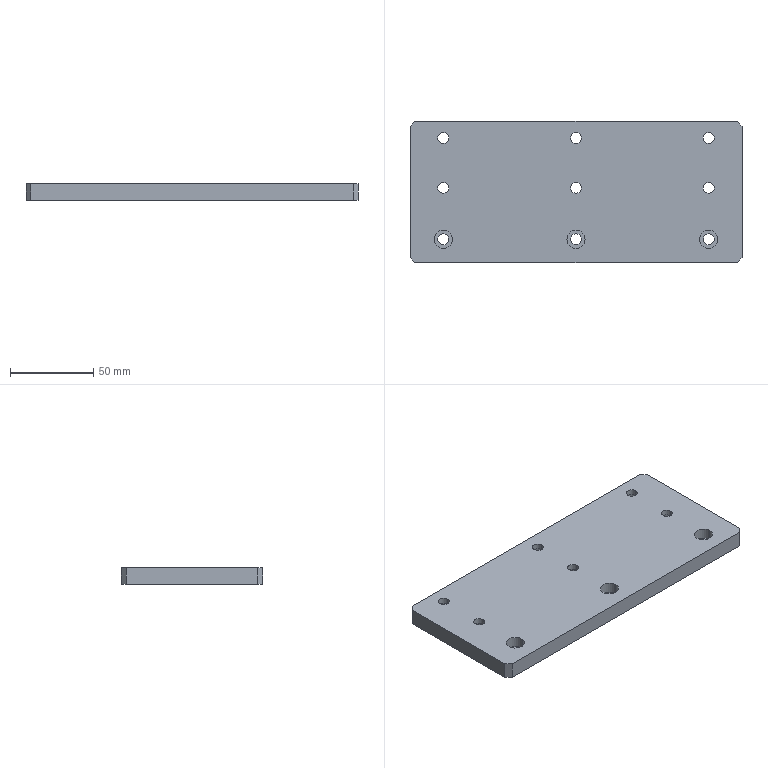Part | SolidWorks | features BaseBody 1 | 1 solid | 55 faces | box 200 x 85 x 10 mm | volume 163128 mm3 | cylinder 36 | plane 19 | commonest cylinder face diameters 6.6 x18 11 x18